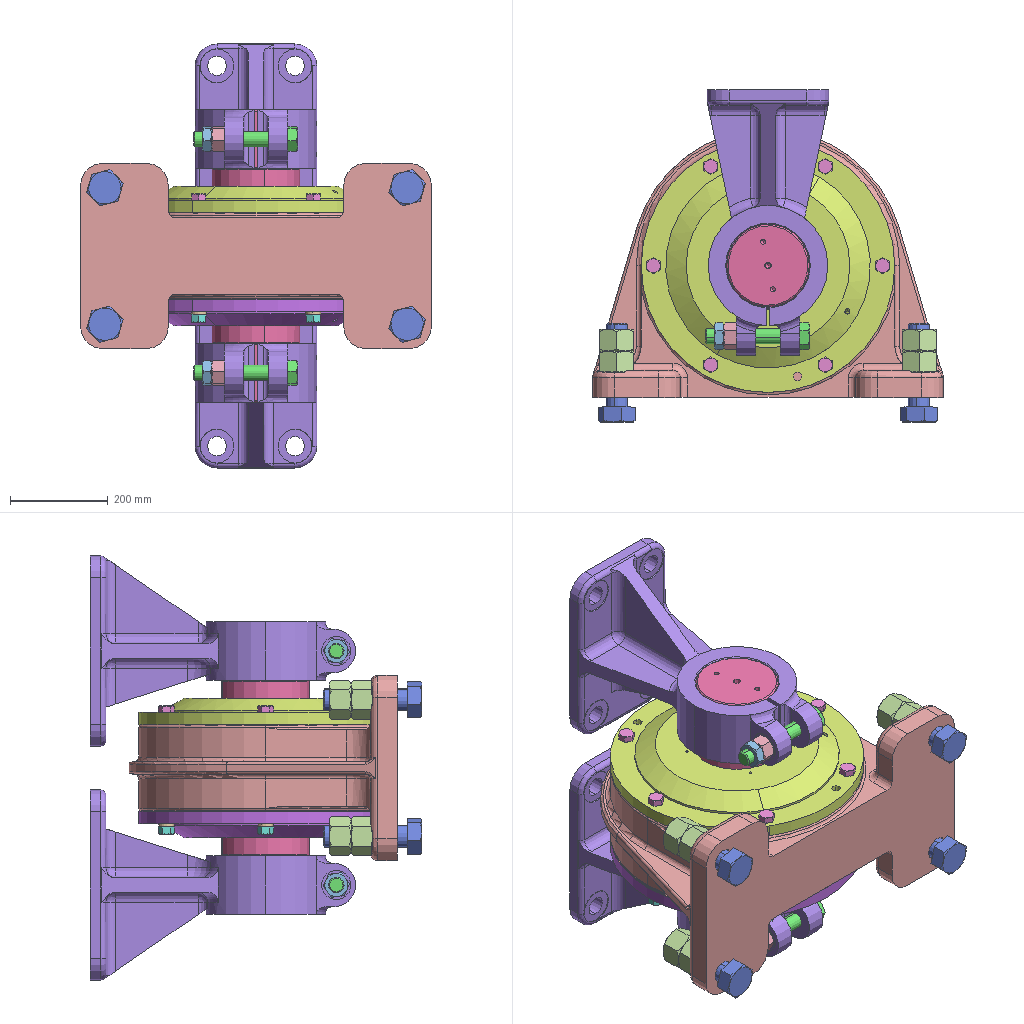Assembly | SolidWorks | 17 different items | 49 placed | box 720 x 680 x 870 mm
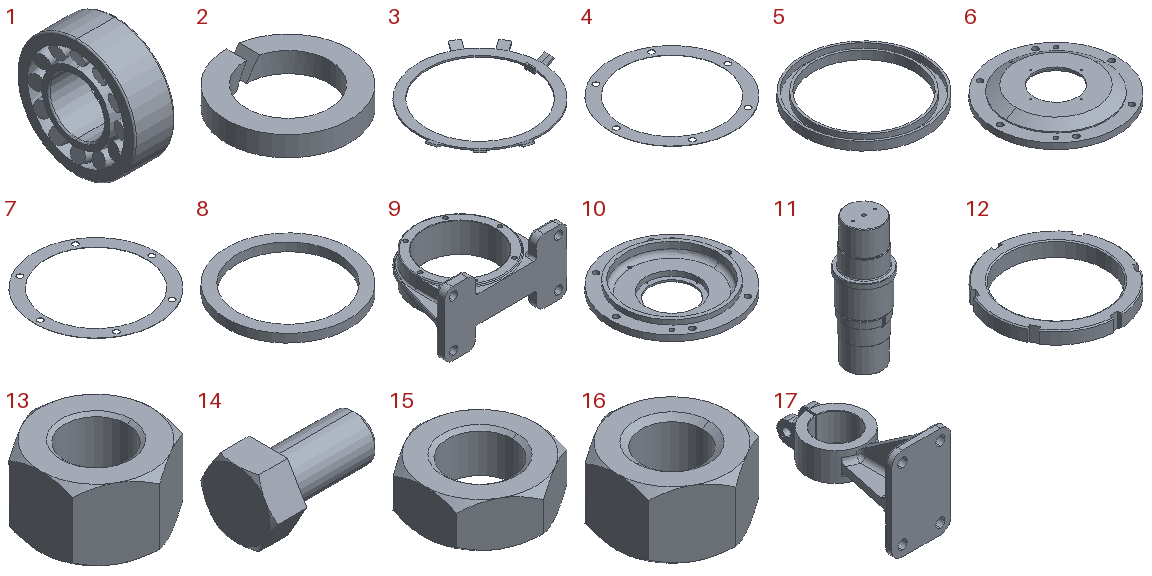Parts list (item | quantity | size | volume | features):
1 | x1 | 102 x 300 x 300 mm | 3829439 mm3 | features Revolution 4, Fillet 2, CirPattern 1, MirrorPattern 1, MirrorSolid 1
2 | x6 | 22.1 x 22.1 x 3.6 mm | 726.172 mm3 | features Cut 1, Extrusion 1
3 | x1 | 223.898 x 212.404 x 8.087 mm | 24578 mm3 | features Boss 1, Cut 1, Revolution 1
4 | x1 | 519 x 519 x 1 mm | 69858 mm3 | features CirPattern 1, Extrusion 1, ICE 1
5 | x1 | 220 x 220 x 15 mm | 105558 mm3 | features Extrusion 1, Shell 1
6 | x1 | 520 x 520 x 74 mm | 4938008 mm3 | features MirrorStock 1
7 | x1 | 519 x 519 x 1 mm | 69858 mm3 | features MirrorStock 1
8 | x1 | 220 x 220 x 15 mm | 105558 mm3 | features MirrorStock 1
9 | x1 | 720 x 550 x 380 mm | 24618968 mm3 | features Fillet 10, ICE 6, Chamfer 1, CirPattern 1, Extrusion 1, LPattern 1
10 | x1 | 520 x 520 x 74 mm | 4938016 mm3 | features CirPattern 3, HoleWzd 2, ICE 2, 3DProfileFeature 1, Fillet 1, Revolution 1
11 | x1 | 220 x 220 x 600 mm | 15781645 mm3 | features ICE 9, Chamfer 4, HoleWzd 3, Fillet 2, Extrusion 1, MirrorPattern 1
12 | x1 | 240 x 239.437 x 30 mm | 460595 mm3 | features Chamfer 3, CirPattern 1, Cut 1, Extrusion 1
13 | x8 | 69.85 x 80.656 x 44.679 mm | 131935 mm3 | features RevCut 4, Extrusion 1, LPattern 1
14 | x12 | 25.857 x 16.483 x 14.275 mm | 2543 mm3 | features RevCut 2, Extrusion 1, Fillet 1, LPattern 1, Revolution 1
15 | x2 | 47.625 x 54.993 x 19.075 mm | 25013 mm3 | features RevCut 4, Extrusion 1, LPattern 1
16 | x8 | 14.275 x 16.483 x 8.56 mm | 1065 mm3 | features RevCut 4, Extrusion 1, LPattern 1
17 | x2 | 250 x 545 x 390 mm | 8795912 mm3 | features ICE 9, Fillet 7, Chamfer 1, Extrusion 1, LPattern 1
Mates (type | each side: item.copy, entity, surface, feature):
Coincident | 9.1 plane | assembly plane | 3 times
Coincident | 1.1 plane | assembly plane
Concentric | 9.1 face cylinder Boss-Extrude1 | 1.1 face cylinder Revolve3
Coincident | 1.1 face plane Revolve1 | 11.1 face plane Boss-Extrude2
Concentric | 1.1 face cylinder Revolve1 | 11.1 face cylinder Boss-Extrude1
Coincident | 1.1 face plane Revolve1 | 3.1 face plane Base-Extrude
Concentric | 3.1 face cylinder Cut-Extrude | 11.1 face cylinder Boss-Extrude5
Coincident | 3.1 face plane Base-Extrude | 12.1 face plane Base-Extrude
Concentric | 11.1 face cylinder Boss-Extrude5 | 12.1 face cylinder Base-Extrude
Coincident | 10.1 face plane Revolve1 | 5.1 face plane Boss-Extrude1
Concentric | 10.1 face cylinder Revolve1 | 5.1 face cylinder Boss-Extrude1
Coincident | 10.1 face plane Revolve1 | 4.1 face plane Boss-Extrude1
Concentric | 10.1 face cylinder Revolve1 | 4.1 face cylinder Boss-Extrude1
Concentric | 10.1 face cylinder CirPattern2 | 4.1 face cylinder CirPattern1
Coincident | 1.1 face plane Revolve3 | 10.1 face plane Revolve1
Concentric | 11.1 face cylinder Boss-Extrude6 | 10.1 face cylinder Revolve1
Concentric | 9.1 face cylinder CirPattern1 | 10.1 face cylinder CirPattern2
Concentric | 9.1 face cylinder LPattern1 | 14.1 face cylinder BaseBody
DistanceDim | 14.1 face plane BaseHead | 9.1 face plane Boss-Extrude2
Coincident | 9.1 face plane LPattern1 | 13.1 face plane BaseNut
Concentric | 14.1 face cylinder BaseBody | 13.1 face cylinder BaseNut
Coincident | 13.1 face plane BaseNut | 13.2 face plane BaseNut
Concentric | 14.1 face cylinder BaseBody | 13.2 face cylinder BaseNut
Coincident | 6.1 face | 14.2 face plane BaseHead
Concentric | 6.1 face | 14.2 face cylinder BaseBody
Coincident | 10.1 face plane Revolve1 | 2.1 face plane Base-Extrude
Concentric | 14.2 face cylinder BaseBody | 2.1 face cylinder Base-Extrude
Coincident | 16.1 face plane BaseNut | 2.1 face plane Base-Extrude
Concentric | 14.2 face cylinder BaseBody | 16.1 face cylinder BaseNut
Coincident | 11.1 face plane Boss-Extrude3 | 17.1 face plane Boss-Extrude1
Concentric | 11.1 face cylinder Boss-Extrude8 | 17.1 face cylinder Boss-Extrude1
Coincident | 17.1 face plane Cut-Extrude2 | 14.3 face plane BaseHead
Concentric | 17.1 face cylinder Boss-Extrude5 | 14.3 face cylinder BaseBody
Coincident | 17.1 face plane Cut-Extrude1 | 16.2 face plane BaseNut
Concentric | 14.3 face cylinder BaseBody | 16.2 face cylinder BaseNut
Coincident | 16.2 face plane BaseNut | 15.1 face plane BaseNut
Concentric | 14.3 face cylinder BaseBody | 15.1 face cylinder BaseNut
Parallel | 17.1 face plane Boss-Extrude2 | assembly plane